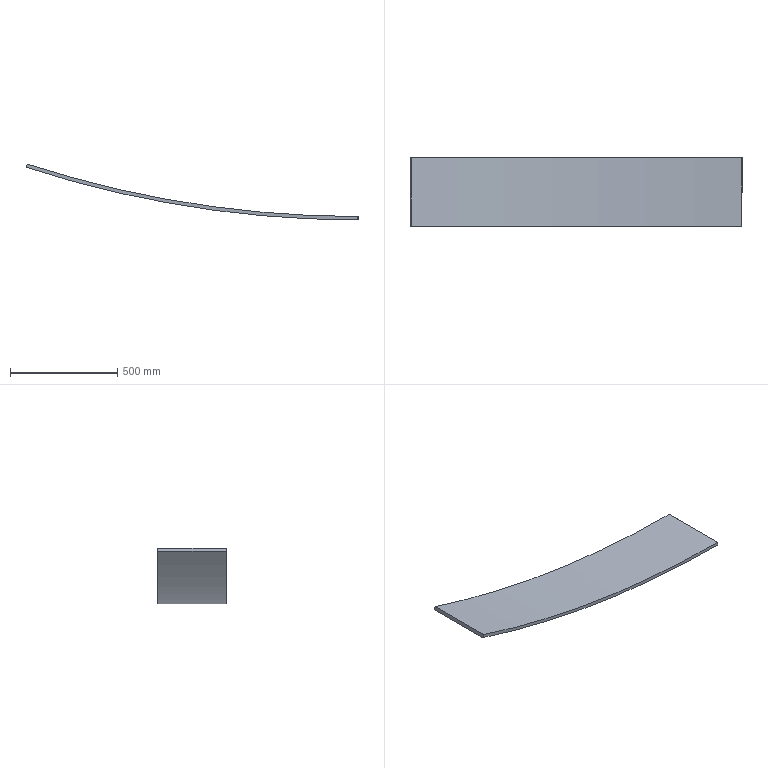Part | SolidWorks | features FlatPattern 1, SM3dBend 1, SMBaseFlange 1, SheetMetal 1 | 1 solid | 14 faces | box 1551 x 320 x 260.824 mm | volume 8058880 mm3 | plane 12 | cylinder 2 | commonest cylinder face diameters 10000 x1 10032 x1
STEP:
#1=CARTESIAN_POINT('',(28.57,320.,244.717));
#2=VERTEX_POINT('',#1);
#3=CARTESIAN_POINT('',(28.242,320.,244.824));
#4=VERTEX_POINT('',#3);
#5=CARTESIAN_POINT('',(28.242,320.,244.824));
#6=DIRECTION('',(-0.9511,0.,0.309));
#7=VECTOR('',#6,1000.);
#8=LINE('',#5,#7);
#9=EDGE_CURVE('',#2,#4,#8,.T.);
#10=ORIENTED_EDGE('',*,*,#9,.F.);
#11=CARTESIAN_POINT('',(23.626,320.,229.501));
#12=VERTEX_POINT('',#11);
#13=CARTESIAN_POINT('',(23.626,320.,229.501));
#14=DIRECTION('',(-0.309,0.,-0.9511));
#15=VECTOR('',#14,1000.);
#16=LINE('',#13,#15);
#17=EDGE_CURVE('',#2,#12,#16,.T.);
#18=ORIENTED_EDGE('',*,*,#17,.T.);
#19=CARTESIAN_POINT('',(23.297,320.,229.607));
#20=VERTEX_POINT('',#19);
#21=CARTESIAN_POINT('',(23.297,320.,229.607));
#22=DIRECTION('',(-0.9511,0.,0.309));
#23=VECTOR('',#22,1000.);
#24=LINE('',#21,#23);
#25=EDGE_CURVE('',#12,#20,#24,.T.);
#26=ORIENTED_EDGE('',*,*,#25,.T.);
#27=CARTESIAN_POINT('',(23.297,320.,229.607));
#28=DIRECTION('',(0.309,0.,0.9511));
#29=VECTOR('',#28,1000.);
#30=LINE('',#27,#29);
#31=EDGE_CURVE('',#20,#4,#30,.T.);
#32=ORIENTED_EDGE('',*,*,#31,.T.);
#33=EDGE_LOOP('',(#10,#18,#26,#32));
#34=FACE_OUTER_BOUND('',#33,.T.);
#35=CARTESIAN_POINT('',(23.297,320.,229.607));
#36=DIRECTION('',(0.,1.,0.));
#37=DIRECTION('',(0.309,0.,0.9511));
#38=AXIS2_PLACEMENT_3D('',#35,#36,#37);
#39=PLANE('',#38);
#40=ADVANCED_FACE('',(#34),#39,.T.);
#41=CARTESIAN_POINT('',(23.297,0.,229.607));
#42=VERTEX_POINT('',#41);
#43=CARTESIAN_POINT('',(23.626,0.,229.501));
#44=VERTEX_POINT('',#43);
#45=CARTESIAN_POINT('',(23.297,0.,229.607));
#46=DIRECTION('',(0.9511,0.,-0.309));
#47=VECTOR('',#46,1000.);
#48=LINE('',#45,#47);
#49=EDGE_CURVE('',#42,#44,#48,.T.);
#50=ORIENTED_EDGE('',*,*,#49,.T.);
#51=CARTESIAN_POINT('',(28.57,0.,244.717));
#52=VERTEX_POINT('',#51);
#53=CARTESIAN_POINT('',(23.626,0.,229.501));
#54=DIRECTION('',(0.309,0.,0.9511));
#55=VECTOR('',#54,1000.);
#56=LINE('',#53,#55);
#57=EDGE_CURVE('',#44,#52,#56,.T.);
#58=ORIENTED_EDGE('',*,*,#57,.T.);
#59=CARTESIAN_POINT('',(28.242,0.,244.824));
#60=VERTEX_POINT('',#59);
#61=CARTESIAN_POINT('',(28.242,0.,244.824));
#62=DIRECTION('',(0.9511,0.,-0.309));
#63=VECTOR('',#62,1000.);
#64=LINE('',#61,#63);
#65=EDGE_CURVE('',#60,#52,#64,.T.);
#66=ORIENTED_EDGE('',*,*,#65,.F.);
#67=CARTESIAN_POINT('',(23.297,0.,229.607));
#68=DIRECTION('',(0.309,0.,0.9511));
#69=VECTOR('',#68,1000.);
#70=LINE('',#67,#69);
#71=EDGE_CURVE('',#42,#60,#70,.T.);
#72=ORIENTED_EDGE('',*,*,#71,.F.);
#73=EDGE_LOOP('',(#50,#58,#66,#72));
#74=FACE_OUTER_BOUND('',#73,.T.);
#75=CARTESIAN_POINT('',(23.297,0.,229.607));
#76=DIRECTION('',(0.,-1.,0.));
#77=DIRECTION('',(-0.309,0.,-0.9511));
#78=AXIS2_PLACEMENT_3D('',#75,#76,#77);
#79=PLANE('',#78);
#80=ADVANCED_FACE('',(#74),#79,.T.);
#81=ORIENTED_EDGE('',*,*,#25,.F.);
#82=CARTESIAN_POINT('',(23.626,320.,229.501));
#83=DIRECTION('',(0.,-1.,0.));
#84=VECTOR('',#83,1000.);
#85=LINE('',#82,#84);
#86=EDGE_CURVE('',#12,#44,#85,.T.);
#87=ORIENTED_EDGE('',*,*,#86,.T.);
#88=ORIENTED_EDGE('',*,*,#49,.F.);
#89=CARTESIAN_POINT('',(23.297,0.,229.607));
#90=DIRECTION('',(0.,-1.,0.));
#91=VECTOR('',#90,1000.);
#92=LINE('',#89,#91);
#93=EDGE_CURVE('',#20,#42,#92,.T.);
#94=ORIENTED_EDGE('',*,*,#93,.F.);
#95=EDGE_LOOP('',(#81,#87,#88,#94));
#96=FACE_OUTER_BOUND('',#95,.T.);
#97=CARTESIAN_POINT('',(23.297,320.,229.607));
#98=DIRECTION('',(-0.309,0.,-0.9511));
#99=DIRECTION('',(-0.9511,0.,0.309));
#100=AXIS2_PLACEMENT_3D('',#97,#98,#99);
#101=PLANE('',#100);
#102=ADVANCED_FACE('',(#96),#101,.T.);
#103=CARTESIAN_POINT('',(28.242,0.,244.824));
#104=DIRECTION('',(0.,-1.,0.));
#105=VECTOR('',#104,1000.);
#106=LINE('',#103,#105);
#107=EDGE_CURVE('',#4,#60,#106,.T.);
#108=ORIENTED_EDGE('',*,*,#107,.F.);
#109=ORIENTED_EDGE('',*,*,#31,.F.);
#110=ORIENTED_EDGE('',*,*,#93,.T.);
#111=ORIENTED_EDGE('',*,*,#71,.T.);
#112=EDGE_LOOP('',(#108,#109,#110,#111));
#113=FACE_OUTER_BOUND('',#112,.T.);
#114=CARTESIAN_POINT('',(23.297,0.,229.607));
#115=DIRECTION('',(-0.9511,0.,0.309));
#116=DIRECTION('',(0.309,0.,0.9511));
#117=AXIS2_PLACEMENT_3D('',#114,#115,#116);
#118=PLANE('',#117);
#119=ADVANCED_FACE('',(#113),#118,.T.);
#120=CARTESIAN_POINT('',(28.57,320.,244.717));
#121=DIRECTION('',(0.,-1.,0.));
#122=VECTOR('',#121,1000.);
#123=LINE('',#120,#122);
#124=EDGE_CURVE('',#2,#52,#123,.T.);
#125=ORIENTED_EDGE('',*,*,#124,.F.);
#126=ORIENTED_EDGE('',*,*,#9,.T.);
#127=ORIENTED_EDGE('',*,*,#107,.T.);
#128=ORIENTED_EDGE('',*,*,#65,.T.);
#129=EDGE_LOOP('',(#125,#126,#127,#128));
#130=FACE_OUTER_BOUND('',#129,.T.);
#131=CARTESIAN_POINT('',(28.242,320.,244.824));
#132=DIRECTION('',(-0.309,0.,-0.9511));
#133=DIRECTION('',(-0.9511,0.,0.309));
#134=AXIS2_PLACEMENT_3D('',#131,#132,#133);
#135=PLANE('',#134);
#136=ADVANCED_FACE('',(#130),#135,.F.);
#137=CARTESIAN_POINT('',(1574.,0.,0.));
#138=VERTEX_POINT('',#137);
#139=CARTESIAN_POINT('',(1574.,320.,0.));
#140=VERTEX_POINT('',#139);
#141=CARTESIAN_POINT('',(1574.,0.,0.));
#142=DIRECTION('',(0.,1.,0.));
#143=VECTOR('',#142,1000.);
#144=LINE('',#141,#143);
#145=EDGE_CURVE('',#138,#140,#144,.T.);
#146=ORIENTED_EDGE('',*,*,#145,.F.);
#147=CARTESIAN_POINT('',(1574.,0.,-16.));
#148=VERTEX_POINT('',#147);
#149=CARTESIAN_POINT('',(1574.,0.,-16.));
#150=DIRECTION('',(0.,0.,1.));
#151=VECTOR('',#150,1000.);
#152=LINE('',#149,#151);
#153=EDGE_CURVE('',#148,#138,#152,.T.);
#154=ORIENTED_EDGE('',*,*,#153,.F.);
#155=CARTESIAN_POINT('',(1574.,320.,-16.));
#156=VERTEX_POINT('',#155);
#157=CARTESIAN_POINT('',(1574.,0.,-16.));
#158=DIRECTION('',(0.,1.,0.));
#159=VECTOR('',#158,1000.);
#160=LINE('',#157,#159);
#161=EDGE_CURVE('',#148,#156,#160,.T.);
#162=ORIENTED_EDGE('',*,*,#161,.T.);
#163=CARTESIAN_POINT('',(1574.,320.,-16.));
#164=DIRECTION('',(0.,0.,1.));
#165=VECTOR('',#164,1000.);
#166=LINE('',#163,#165);
#167=EDGE_CURVE('',#156,#140,#166,.T.);
#168=ORIENTED_EDGE('',*,*,#167,.T.);
#169=EDGE_LOOP('',(#146,#154,#162,#168));
#170=FACE_OUTER_BOUND('',#169,.T.);
#171=CARTESIAN_POINT('',(1574.,0.,-16.));
#172=DIRECTION('',(1.,0.,0.));
#173=DIRECTION('',(0.,1.,0.));
#174=AXIS2_PLACEMENT_3D('',#171,#172,#173);
#175=PLANE('',#174);
#176=ADVANCED_FACE('',(#170),#175,.T.);
#177=CARTESIAN_POINT('',(1573.655,320.,-16.));
#178=VERTEX_POINT('',#177);
#179=CARTESIAN_POINT('',(1573.655,0.,-16.));
#180=VERTEX_POINT('',#179);
#181=CARTESIAN_POINT('',(1573.655,320.,-16.));
#182=DIRECTION('',(0.,-1.,0.));
#183=VECTOR('',#182,1000.);
#184=LINE('',#181,#183);
#185=EDGE_CURVE('',#178,#180,#184,.T.);
#186=ORIENTED_EDGE('',*,*,#185,.F.);
#187=CARTESIAN_POINT('',(0.,320.,-16.));
#188=DIRECTION('',(-1.,0.,0.));
#189=VECTOR('',#188,1000.);
#190=LINE('',#187,#189);
#191=EDGE_CURVE('',#156,#178,#190,.T.);
#192=ORIENTED_EDGE('',*,*,#191,.F.);
#193=ORIENTED_EDGE('',*,*,#161,.F.);
#194=CARTESIAN_POINT('',(0.,0.,-16.));
#195=DIRECTION('',(1.,0.,0.));
#196=VECTOR('',#195,1000.);
#197=LINE('',#194,#196);
#198=EDGE_CURVE('',#180,#148,#197,.T.);
#199=ORIENTED_EDGE('',*,*,#198,.F.);
#200=EDGE_LOOP('',(#186,#192,#193,#199));
#201=FACE_OUTER_BOUND('',#200,.T.);
#202=CARTESIAN_POINT('',(0.,320.,-16.));
#203=DIRECTION('',(0.,0.,-1.));
#204=DIRECTION('',(-1.,0.,0.));
#205=AXIS2_PLACEMENT_3D('',#202,#203,#204);
#206=PLANE('',#205);
#207=ADVANCED_FACE('',(#201),#206,.T.);
#208=CARTESIAN_POINT('',(1573.655,320.,0.));
#209=VERTEX_POINT('',#208);
#210=CARTESIAN_POINT('',(1573.655,320.,-16.));
#211=DIRECTION('',(0.,0.,-1.));
#212=VECTOR('',#211,1000.);
#213=LINE('',#210,#212);
#214=EDGE_CURVE('',#209,#178,#213,.T.);
#215=ORIENTED_EDGE('',*,*,#214,.F.);
#216=CARTESIAN_POINT('',(0.,320.,0.));
#217=DIRECTION('',(-1.,0.,0.));
#218=VECTOR('',#217,1000.);
#219=LINE('',#216,#218);
#220=EDGE_CURVE('',#140,#209,#219,.T.);
#221=ORIENTED_EDGE('',*,*,#220,.F.);
#222=ORIENTED_EDGE('',*,*,#167,.F.);
#223=ORIENTED_EDGE('',*,*,#191,.T.);
#224=EDGE_LOOP('',(#215,#221,#222,#223));
#225=FACE_OUTER_BOUND('',#224,.T.);
#226=CARTESIAN_POINT('',(0.,320.,-16.));
#227=DIRECTION('',(0.,1.,0.));
#228=DIRECTION('',(0.,0.,1.));
#229=AXIS2_PLACEMENT_3D('',#226,#227,#228);
#230=PLANE('',#229);
#231=ADVANCED_FACE('',(#225),#230,.T.);
#232=ORIENTED_EDGE('',*,*,#220,.T.);
#233=CARTESIAN_POINT('',(1573.655,0.,0.));
#234=VERTEX_POINT('',#233);
#235=CARTESIAN_POINT('',(1573.655,320.,0.));
#236=DIRECTION('',(0.,-1.,0.));
#237=VECTOR('',#236,1000.);
#238=LINE('',#235,#237);
#239=EDGE_CURVE('',#209,#234,#238,.T.);
#240=ORIENTED_EDGE('',*,*,#239,.T.);
#241=CARTESIAN_POINT('',(0.,0.,0.));
#242=DIRECTION('',(1.,0.,0.));
#243=VECTOR('',#242,1000.);
#244=LINE('',#241,#243);
#245=EDGE_CURVE('',#234,#138,#244,.T.);
#246=ORIENTED_EDGE('',*,*,#245,.T.);
#247=ORIENTED_EDGE('',*,*,#145,.T.);
#248=EDGE_LOOP('',(#232,#240,#246,#247));
#249=FACE_OUTER_BOUND('',#248,.T.);
#250=CARTESIAN_POINT('',(0.,320.,0.));
#251=DIRECTION('',(0.,0.,-1.));
#252=DIRECTION('',(-1.,0.,0.));
#253=AXIS2_PLACEMENT_3D('',#250,#251,#252);
#254=PLANE('',#253);
#255=ADVANCED_FACE('',(#249),#254,.F.);
#256=CARTESIAN_POINT('',(1573.655,0.,-16.));
#257=DIRECTION('',(0.,0.,1.));
#258=VECTOR('',#257,1000.);
#259=LINE('',#256,#258);
#260=EDGE_CURVE('',#180,#234,#259,.T.);
#261=ORIENTED_EDGE('',*,*,#260,.F.);
#262=ORIENTED_EDGE('',*,*,#198,.T.);
#263=ORIENTED_EDGE('',*,*,#153,.T.);
#264=ORIENTED_EDGE('',*,*,#245,.F.);
#265=EDGE_LOOP('',(#261,#262,#263,#264));
#266=FACE_OUTER_BOUND('',#265,.T.);
#267=CARTESIAN_POINT('',(0.,0.,-16.));
#268=DIRECTION('',(0.,-1.,0.));
#269=DIRECTION('',(0.,0.,-1.));
#270=AXIS2_PLACEMENT_3D('',#267,#268,#269);
#271=PLANE('',#270);
#272=ADVANCED_FACE('',(#266),#271,.T.);
#273=ORIENTED_EDGE('',*,*,#17,.F.);
#274=CARTESIAN_POINT('',(1573.655,320.,5000.));
#275=DIRECTION('',(0.,-1.,0.));
#276=DIRECTION('',(-1.,0.,0.));
#277=AXIS2_PLACEMENT_3D('',#274,#275,#276);
#278=CIRCLE('',#277,5000.);
#279=EDGE_CURVE('',#2,#209,#278,.T.);
#280=ORIENTED_EDGE('',*,*,#279,.T.);
#281=ORIENTED_EDGE('',*,*,#214,.T.);
#282=CARTESIAN_POINT('',(1573.655,320.,5000.));
#283=DIRECTION('',(0.,-1.,0.));
#284=DIRECTION('',(-1.,0.,0.));
#285=AXIS2_PLACEMENT_3D('',#282,#283,#284);
#286=CIRCLE('',#285,5016.);
#287=EDGE_CURVE('',#12,#178,#286,.T.);
#288=ORIENTED_EDGE('',*,*,#287,.F.);
#289=EDGE_LOOP('',(#273,#280,#281,#288));
#290=FACE_OUTER_BOUND('',#289,.T.);
#291=CARTESIAN_POINT('',(1573.655,320.,5000.));
#292=DIRECTION('',(0.,1.,0.));
#293=DIRECTION('',(-1.,0.,0.));
#294=AXIS2_PLACEMENT_3D('',#291,#292,#293);
#295=PLANE('',#294);
#296=ADVANCED_FACE('',(#290),#295,.T.);
#297=ORIENTED_EDGE('',*,*,#185,.T.);
#298=CARTESIAN_POINT('',(1573.655,0.,5000.));
#299=DIRECTION('',(0.,1.,0.));
#300=DIRECTION('',(1.,0.,0.));
#301=AXIS2_PLACEMENT_3D('',#298,#299,#300);
#302=CIRCLE('',#301,5016.);
#303=EDGE_CURVE('',#180,#44,#302,.T.);
#304=ORIENTED_EDGE('',*,*,#303,.T.);
#305=ORIENTED_EDGE('',*,*,#86,.F.);
#306=ORIENTED_EDGE('',*,*,#287,.T.);
#307=EDGE_LOOP('',(#297,#304,#305,#306));
#308=FACE_OUTER_BOUND('',#307,.T.);
#309=CARTESIAN_POINT('',(1573.655,-1445.602,5000.));
#310=DIRECTION('',(0.,1.,0.));
#311=DIRECTION('',(-1.,0.,0.));
#312=AXIS2_PLACEMENT_3D('',#309,#310,#311);
#313=CYLINDRICAL_SURFACE('',#312,5016.);
#314=ADVANCED_FACE('',(#308),#313,.T.);
#315=CARTESIAN_POINT('',(1573.655,0.,5000.));
#316=DIRECTION('',(0.,1.,0.));
#317=DIRECTION('',(-1.,0.,0.));
#318=AXIS2_PLACEMENT_3D('',#315,#316,#317);
#319=CIRCLE('',#318,5000.);
#320=EDGE_CURVE('',#234,#52,#319,.T.);
#321=ORIENTED_EDGE('',*,*,#320,.T.);
#322=ORIENTED_EDGE('',*,*,#57,.F.);
#323=ORIENTED_EDGE('',*,*,#303,.F.);
#324=ORIENTED_EDGE('',*,*,#260,.T.);
#325=EDGE_LOOP('',(#321,#322,#323,#324));
#326=FACE_OUTER_BOUND('',#325,.T.);
#327=CARTESIAN_POINT('',(1573.655,0.,5000.));
#328=DIRECTION('',(0.,-1.,0.));
#329=DIRECTION('',(1.,0.,0.));
#330=AXIS2_PLACEMENT_3D('',#327,#328,#329);
#331=PLANE('',#330);
#332=ADVANCED_FACE('',(#326),#331,.T.);
#333=ORIENTED_EDGE('',*,*,#239,.F.);
#334=ORIENTED_EDGE('',*,*,#279,.F.);
#335=ORIENTED_EDGE('',*,*,#124,.T.);
#336=ORIENTED_EDGE('',*,*,#320,.F.);
#337=EDGE_LOOP('',(#333,#334,#335,#336));
#338=FACE_OUTER_BOUND('',#337,.T.);
#339=CARTESIAN_POINT('',(1573.655,-1445.602,5000.));
#340=DIRECTION('',(0.,1.,0.));
#341=DIRECTION('',(-1.,0.,0.));
#342=AXIS2_PLACEMENT_3D('',#339,#340,#341);
#343=CYLINDRICAL_SURFACE('',#342,5000.);
#344=ADVANCED_FACE('',(#338),#343,.F.);
#345=CLOSED_SHELL('',(#40,#80,#102,#119,#136,#176,#207,#231,#255,#272,#296,#314,#332,#344));
#346=MANIFOLD_SOLID_BREP('',#345);
#347=CARTESIAN_POINT('',(0.,0.,0.));
#348=DIRECTION('',(0.,0.,1.));
#349=DIRECTION('',(1.,0.,0.));
#350=AXIS2_PLACEMENT_3D('',#347,#348,#349);
#351=(LENGTH_UNIT()NAMED_UNIT(*)SI_UNIT(.MILLI.,.METRE.));
#352=UNCERTAINTY_MEASURE_WITH_UNIT(LENGTH_MEASURE(0.00001),#351,'','');
#353=(NAMED_UNIT(*)PLANE_ANGLE_UNIT()SI_UNIT($,.RADIAN.));
#354=(NAMED_UNIT(*)SI_UNIT($,.STERADIAN.)SOLID_ANGLE_UNIT());
#355=(GEOMETRIC_REPRESENTATION_CONTEXT(3)GLOBAL_UNCERTAINTY_ASSIGNED_CONTEXT((#352))GLOBAL_UNIT_ASSIGNED_CONTEXT((#351,#353,#354))REPRESENTATION_CONTEXT('',''));
#356=ADVANCED_BREP_SHAPE_REPRESENTATION('',(#346,#350),#355);